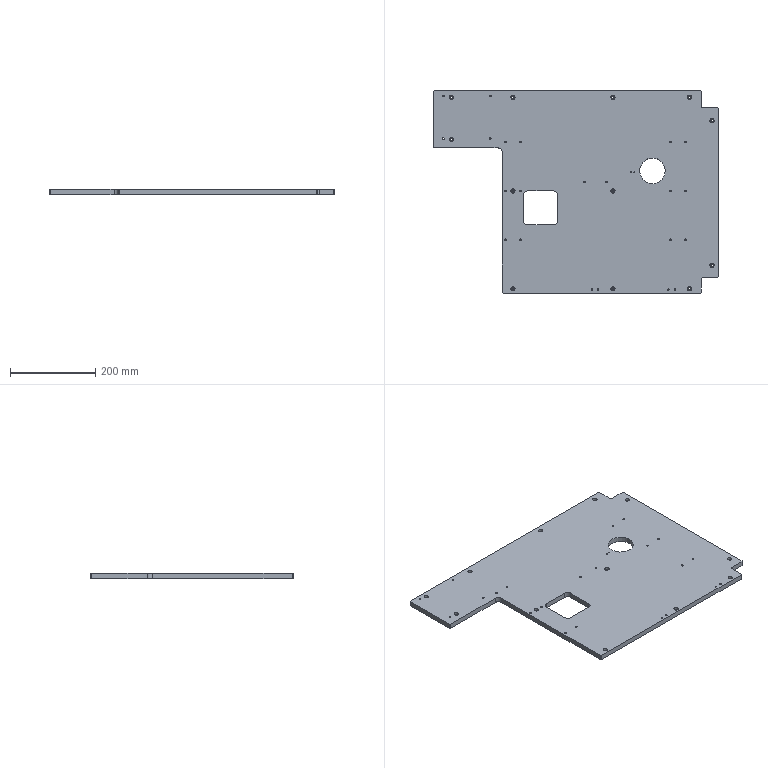Part | STEP file | FBDS-TB | 1 solid | 144 faces | box 669.5 x 475 x 12 mm | volume 2998204 mm3 | cylinder 105 | plane 35 | cone 4 | commonest cylinder face diameters 4.2 x36 10 x26 5.5 x24 3.3 x8 20 x5 2.5 x4